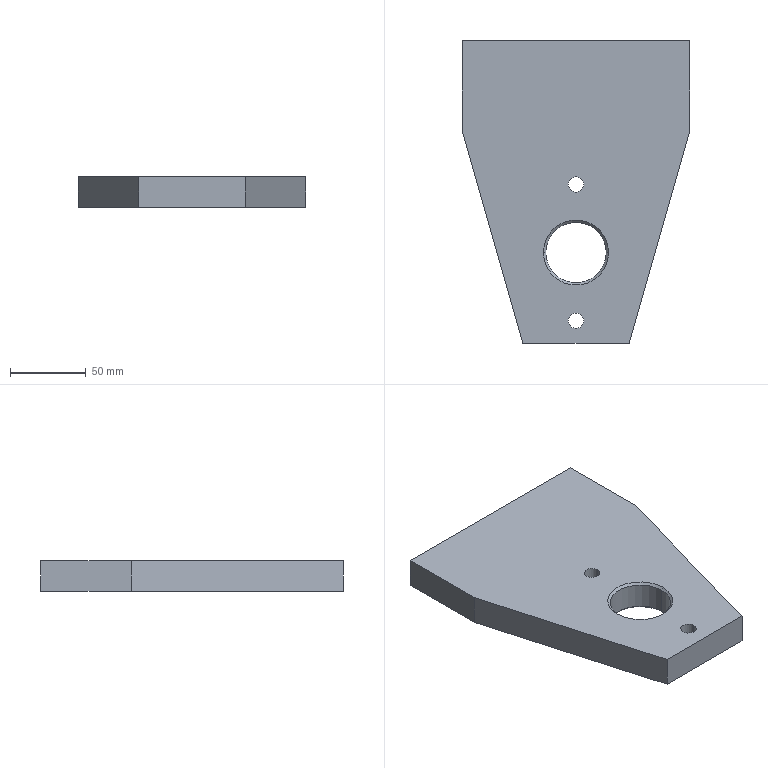Part | SolidWorks | features Chamfer 1, Extrusion 1, HoleWzd 1 | 1 solid | 18 faces | box 150 x 200 x 20 mm | volume 459309 mm3 | plane 8 | cylinder 6 | cone 4 | commonest cylinder face diameters 10.2 x4 40 x2
STEP:
#1=CARTESIAN_POINT('',(55.,-140.,18.5));
#2=VERTEX_POINT('',#1);
#3=CARTESIAN_POINT('',(95.,-140.,18.5));
#4=VERTEX_POINT('',#3);
#5=CARTESIAN_POINT('',(75.,-140.,18.5));
#6=DIRECTION('',(0.,0.,1.));
#7=DIRECTION('',(-1.,0.,0.));
#8=AXIS2_PLACEMENT_3D('',#5,#6,#7);
#9=CIRCLE('',#8,20.);
#10=EDGE_CURVE('',#2,#4,#9,.T.);
#11=ORIENTED_EDGE('',*,*,#10,.F.);
#12=CARTESIAN_POINT('',(53.5,-140.,20.));
#13=VERTEX_POINT('',#12);
#14=CARTESIAN_POINT('',(55.,-140.,18.5));
#15=DIRECTION('',(-0.7071,0.,0.7071));
#16=VECTOR('',#15,1000.);
#17=LINE('',#14,#16);
#18=EDGE_CURVE('',#2,#13,#17,.T.);
#19=ORIENTED_EDGE('',*,*,#18,.T.);
#20=CARTESIAN_POINT('',(96.5,-140.,20.));
#21=VERTEX_POINT('',#20);
#22=CARTESIAN_POINT('',(75.,-140.,20.));
#23=DIRECTION('',(0.,0.,-1.));
#24=DIRECTION('',(-1.,0.,0.));
#25=AXIS2_PLACEMENT_3D('',#22,#23,#24);
#26=CIRCLE('',#25,21.5);
#27=EDGE_CURVE('',#21,#13,#26,.T.);
#28=ORIENTED_EDGE('',*,*,#27,.F.);
#29=CARTESIAN_POINT('',(95.,-140.,18.5));
#30=DIRECTION('',(0.7071,0.,0.7071));
#31=VECTOR('',#30,1000.);
#32=LINE('',#29,#31);
#33=EDGE_CURVE('',#4,#21,#32,.T.);
#34=ORIENTED_EDGE('',*,*,#33,.F.);
#35=EDGE_LOOP('',(#11,#19,#28,#34));
#36=FACE_OUTER_BOUND('',#35,.T.);
#37=CARTESIAN_POINT('',(75.,-140.,18.5));
#38=DIRECTION('',(0.,0.,1.));
#39=DIRECTION('',(1.,0.,0.));
#40=AXIS2_PLACEMENT_3D('',#37,#38,#39);
#41=CONICAL_SURFACE('',#40,20.,0.7854);
#42=ADVANCED_FACE('',(#36),#41,.F.);
#43=CARTESIAN_POINT('',(95.,-140.,1.5));
#44=VERTEX_POINT('',#43);
#45=CARTESIAN_POINT('',(55.,-140.,1.5));
#46=VERTEX_POINT('',#45);
#47=CARTESIAN_POINT('',(75.,-140.,1.5));
#48=DIRECTION('',(0.,0.,-1.));
#49=DIRECTION('',(-1.,0.,0.));
#50=AXIS2_PLACEMENT_3D('',#47,#48,#49);
#51=CIRCLE('',#50,20.);
#52=EDGE_CURVE('',#44,#46,#51,.T.);
#53=ORIENTED_EDGE('',*,*,#52,.F.);
#54=CARTESIAN_POINT('',(96.5,-140.,0.));
#55=VERTEX_POINT('',#54);
#56=CARTESIAN_POINT('',(96.5,-140.,0.));
#57=DIRECTION('',(0.7071,0.,-0.7071));
#58=VECTOR('',#57,1000.);
#59=LINE('',#56,#58);
#60=EDGE_CURVE('',#44,#55,#59,.T.);
#61=ORIENTED_EDGE('',*,*,#60,.T.);
#62=CARTESIAN_POINT('',(53.5,-140.,0.));
#63=VERTEX_POINT('',#62);
#64=CARTESIAN_POINT('',(75.,-140.,0.));
#65=DIRECTION('',(0.,0.,1.));
#66=DIRECTION('',(-1.,0.,0.));
#67=AXIS2_PLACEMENT_3D('',#64,#65,#66);
#68=CIRCLE('',#67,21.5);
#69=EDGE_CURVE('',#63,#55,#68,.T.);
#70=ORIENTED_EDGE('',*,*,#69,.F.);
#71=CARTESIAN_POINT('',(53.5,-140.,0.));
#72=DIRECTION('',(-0.7071,0.,-0.7071));
#73=VECTOR('',#72,1000.);
#74=LINE('',#71,#73);
#75=EDGE_CURVE('',#46,#63,#74,.T.);
#76=ORIENTED_EDGE('',*,*,#75,.F.);
#77=EDGE_LOOP('',(#53,#61,#70,#76));
#78=FACE_OUTER_BOUND('',#77,.T.);
#79=CARTESIAN_POINT('',(75.,-140.,0.));
#80=DIRECTION('',(0.,0.,-1.));
#81=DIRECTION('',(-1.,0.,0.));
#82=AXIS2_PLACEMENT_3D('',#79,#80,#81);
#83=CONICAL_SURFACE('',#82,21.5,0.7854);
#84=ADVANCED_FACE('',(#78),#83,.F.);
#85=CARTESIAN_POINT('',(80.1,-95.,0.));
#86=VERTEX_POINT('',#85);
#87=CARTESIAN_POINT('',(69.9,-95.,0.));
#88=VERTEX_POINT('',#87);
#89=CARTESIAN_POINT('',(75.,-95.,0.));
#90=DIRECTION('',(0.,0.,-1.));
#91=DIRECTION('',(-1.,0.,0.));
#92=AXIS2_PLACEMENT_3D('',#89,#90,#91);
#93=CIRCLE('',#92,5.1);
#94=EDGE_CURVE('',#86,#88,#93,.T.);
#95=ORIENTED_EDGE('',*,*,#94,.T.);
#96=CARTESIAN_POINT('',(69.9,-95.,20.));
#97=VERTEX_POINT('',#96);
#98=CARTESIAN_POINT('',(69.9,-95.,20.));
#99=DIRECTION('',(0.,0.,1.));
#100=VECTOR('',#99,1000.);
#101=LINE('',#98,#100);
#102=EDGE_CURVE('',#88,#97,#101,.T.);
#103=ORIENTED_EDGE('',*,*,#102,.T.);
#104=CARTESIAN_POINT('',(80.1,-95.,20.));
#105=VERTEX_POINT('',#104);
#106=CARTESIAN_POINT('',(75.,-95.,20.));
#107=DIRECTION('',(0.,0.,1.));
#108=DIRECTION('',(1.,0.,0.));
#109=AXIS2_PLACEMENT_3D('',#106,#107,#108);
#110=CIRCLE('',#109,5.1);
#111=EDGE_CURVE('',#97,#105,#110,.T.);
#112=ORIENTED_EDGE('',*,*,#111,.T.);
#113=CARTESIAN_POINT('',(80.1,-95.,20.));
#114=DIRECTION('',(0.,0.,1.));
#115=VECTOR('',#114,1000.);
#116=LINE('',#113,#115);
#117=EDGE_CURVE('',#86,#105,#116,.T.);
#118=ORIENTED_EDGE('',*,*,#117,.F.);
#119=EDGE_LOOP('',(#95,#103,#112,#118));
#120=FACE_OUTER_BOUND('',#119,.T.);
#121=CARTESIAN_POINT('',(75.,-95.,20.));
#122=DIRECTION('',(0.,0.,1.));
#123=DIRECTION('',(1.,0.,0.));
#124=AXIS2_PLACEMENT_3D('',#121,#122,#123);
#125=CYLINDRICAL_SURFACE('',#124,5.1);
#126=ADVANCED_FACE('',(#120),#125,.F.);
#127=CARTESIAN_POINT('',(80.1,-185.,0.));
#128=VERTEX_POINT('',#127);
#129=CARTESIAN_POINT('',(69.9,-185.,0.));
#130=VERTEX_POINT('',#129);
#131=CARTESIAN_POINT('',(75.,-185.,0.));
#132=DIRECTION('',(0.,0.,-1.));
#133=DIRECTION('',(-1.,0.,0.));
#134=AXIS2_PLACEMENT_3D('',#131,#132,#133);
#135=CIRCLE('',#134,5.1);
#136=EDGE_CURVE('',#128,#130,#135,.T.);
#137=ORIENTED_EDGE('',*,*,#136,.T.);
#138=CARTESIAN_POINT('',(69.9,-185.,20.));
#139=VERTEX_POINT('',#138);
#140=CARTESIAN_POINT('',(69.9,-185.,20.));
#141=DIRECTION('',(0.,0.,1.));
#142=VECTOR('',#141,1000.);
#143=LINE('',#140,#142);
#144=EDGE_CURVE('',#130,#139,#143,.T.);
#145=ORIENTED_EDGE('',*,*,#144,.T.);
#146=CARTESIAN_POINT('',(80.1,-185.,20.));
#147=VERTEX_POINT('',#146);
#148=CARTESIAN_POINT('',(75.,-185.,20.));
#149=DIRECTION('',(0.,0.,1.));
#150=DIRECTION('',(1.,0.,0.));
#151=AXIS2_PLACEMENT_3D('',#148,#149,#150);
#152=CIRCLE('',#151,5.1);
#153=EDGE_CURVE('',#139,#147,#152,.T.);
#154=ORIENTED_EDGE('',*,*,#153,.T.);
#155=CARTESIAN_POINT('',(80.1,-185.,20.));
#156=DIRECTION('',(0.,0.,1.));
#157=VECTOR('',#156,1000.);
#158=LINE('',#155,#157);
#159=EDGE_CURVE('',#128,#147,#158,.T.);
#160=ORIENTED_EDGE('',*,*,#159,.F.);
#161=EDGE_LOOP('',(#137,#145,#154,#160));
#162=FACE_OUTER_BOUND('',#161,.T.);
#163=CARTESIAN_POINT('',(75.,-185.,20.));
#164=DIRECTION('',(0.,0.,1.));
#165=DIRECTION('',(1.,0.,0.));
#166=AXIS2_PLACEMENT_3D('',#163,#164,#165);
#167=CYLINDRICAL_SURFACE('',#166,5.1);
#168=ADVANCED_FACE('',(#162),#167,.F.);
#169=ORIENTED_EDGE('',*,*,#10,.T.);
#170=CARTESIAN_POINT('',(95.,-140.,20.));
#171=DIRECTION('',(0.,0.,-1.));
#172=VECTOR('',#171,1000.);
#173=LINE('',#170,#172);
#174=EDGE_CURVE('',#4,#44,#173,.T.);
#175=ORIENTED_EDGE('',*,*,#174,.T.);
#176=ORIENTED_EDGE('',*,*,#52,.T.);
#177=CARTESIAN_POINT('',(55.,-140.,20.));
#178=DIRECTION('',(0.,0.,-1.));
#179=VECTOR('',#178,1000.);
#180=LINE('',#177,#179);
#181=EDGE_CURVE('',#2,#46,#180,.T.);
#182=ORIENTED_EDGE('',*,*,#181,.F.);
#183=EDGE_LOOP('',(#169,#175,#176,#182));
#184=FACE_OUTER_BOUND('',#183,.T.);
#185=CARTESIAN_POINT('',(75.,-140.,20.));
#186=DIRECTION('',(0.,0.,-1.));
#187=DIRECTION('',(-1.,0.,0.));
#188=AXIS2_PLACEMENT_3D('',#185,#186,#187);
#189=CYLINDRICAL_SURFACE('',#188,20.);
#190=ADVANCED_FACE('',(#184),#189,.F.);
#191=ORIENTED_EDGE('',*,*,#27,.T.);
#192=CARTESIAN_POINT('',(75.,-140.,20.));
#193=DIRECTION('',(0.,0.,-1.));
#194=DIRECTION('',(-1.,0.,0.));
#195=AXIS2_PLACEMENT_3D('',#192,#193,#194);
#196=CIRCLE('',#195,21.5);
#197=EDGE_CURVE('',#13,#21,#196,.T.);
#198=ORIENTED_EDGE('',*,*,#197,.T.);
#199=EDGE_LOOP('',(#191,#198));
#200=FACE_BOUND('',#199,.T.);
#201=CARTESIAN_POINT('',(75.,-95.,20.));
#202=DIRECTION('',(0.,0.,1.));
#203=DIRECTION('',(1.,0.,0.));
#204=AXIS2_PLACEMENT_3D('',#201,#202,#203);
#205=CIRCLE('',#204,5.1);
#206=EDGE_CURVE('',#105,#97,#205,.T.);
#207=ORIENTED_EDGE('',*,*,#206,.F.);
#208=ORIENTED_EDGE('',*,*,#111,.F.);
#209=EDGE_LOOP('',(#207,#208));
#210=FACE_BOUND('',#209,.T.);
#211=CARTESIAN_POINT('',(0.,0.,20.));
#212=VERTEX_POINT('',#211);
#213=CARTESIAN_POINT('',(0.,-60.,20.));
#214=VERTEX_POINT('',#213);
#215=CARTESIAN_POINT('',(0.,-60.,20.));
#216=DIRECTION('',(0.,-1.,0.));
#217=VECTOR('',#216,1000.);
#218=LINE('',#215,#217);
#219=EDGE_CURVE('',#212,#214,#218,.T.);
#220=ORIENTED_EDGE('',*,*,#219,.T.);
#221=CARTESIAN_POINT('',(40.,-200.,20.));
#222=VERTEX_POINT('',#221);
#223=CARTESIAN_POINT('',(40.,-200.,20.));
#224=DIRECTION('',(0.2747,-0.9615,0.));
#225=VECTOR('',#224,1000.);
#226=LINE('',#223,#225);
#227=EDGE_CURVE('',#214,#222,#226,.T.);
#228=ORIENTED_EDGE('',*,*,#227,.T.);
#229=CARTESIAN_POINT('',(110.,-200.,20.));
#230=VERTEX_POINT('',#229);
#231=CARTESIAN_POINT('',(110.,-200.,20.));
#232=DIRECTION('',(1.,0.,0.));
#233=VECTOR('',#232,1000.);
#234=LINE('',#231,#233);
#235=EDGE_CURVE('',#222,#230,#234,.T.);
#236=ORIENTED_EDGE('',*,*,#235,.T.);
#237=CARTESIAN_POINT('',(150.,-60.,20.));
#238=VERTEX_POINT('',#237);
#239=CARTESIAN_POINT('',(150.,-60.,20.));
#240=DIRECTION('',(0.2747,0.9615,0.));
#241=VECTOR('',#240,1000.);
#242=LINE('',#239,#241);
#243=EDGE_CURVE('',#230,#238,#242,.T.);
#244=ORIENTED_EDGE('',*,*,#243,.T.);
#245=CARTESIAN_POINT('',(150.,0.,20.));
#246=VERTEX_POINT('',#245);
#247=CARTESIAN_POINT('',(150.,0.,20.));
#248=DIRECTION('',(0.,1.,0.));
#249=VECTOR('',#248,1000.);
#250=LINE('',#247,#249);
#251=EDGE_CURVE('',#238,#246,#250,.T.);
#252=ORIENTED_EDGE('',*,*,#251,.T.);
#253=CARTESIAN_POINT('',(0.,0.,20.));
#254=DIRECTION('',(-1.,0.,0.));
#255=VECTOR('',#254,1000.);
#256=LINE('',#253,#255);
#257=EDGE_CURVE('',#246,#212,#256,.T.);
#258=ORIENTED_EDGE('',*,*,#257,.T.);
#259=EDGE_LOOP('',(#220,#228,#236,#244,#252,#258));
#260=FACE_OUTER_BOUND('',#259,.T.);
#261=CARTESIAN_POINT('',(75.,-185.,20.));
#262=DIRECTION('',(0.,0.,1.));
#263=DIRECTION('',(1.,0.,0.));
#264=AXIS2_PLACEMENT_3D('',#261,#262,#263);
#265=CIRCLE('',#264,5.1);
#266=EDGE_CURVE('',#147,#139,#265,.T.);
#267=ORIENTED_EDGE('',*,*,#266,.F.);
#268=ORIENTED_EDGE('',*,*,#153,.F.);
#269=EDGE_LOOP('',(#267,#268));
#270=FACE_BOUND('',#269,.T.);
#271=CARTESIAN_POINT('',(0.,0.,20.));
#272=DIRECTION('',(0.,0.,-1.));
#273=DIRECTION('',(-1.,0.,0.));
#274=AXIS2_PLACEMENT_3D('',#271,#272,#273);
#275=PLANE('',#274);
#276=ADVANCED_FACE('',(#200,#210,#260,#270),#275,.F.);
#277=ORIENTED_EDGE('',*,*,#69,.T.);
#278=CARTESIAN_POINT('',(75.,-140.,0.));
#279=DIRECTION('',(0.,0.,1.));
#280=DIRECTION('',(-1.,0.,0.));
#281=AXIS2_PLACEMENT_3D('',#278,#279,#280);
#282=CIRCLE('',#281,21.5);
#283=EDGE_CURVE('',#55,#63,#282,.T.);
#284=ORIENTED_EDGE('',*,*,#283,.T.);
#285=EDGE_LOOP('',(#277,#284));
#286=FACE_BOUND('',#285,.T.);
#287=ORIENTED_EDGE('',*,*,#94,.F.);
#288=CARTESIAN_POINT('',(75.,-95.,0.));
#289=DIRECTION('',(0.,0.,-1.));
#290=DIRECTION('',(-1.,0.,0.));
#291=AXIS2_PLACEMENT_3D('',#288,#289,#290);
#292=CIRCLE('',#291,5.1);
#293=EDGE_CURVE('',#88,#86,#292,.T.);
#294=ORIENTED_EDGE('',*,*,#293,.F.);
#295=EDGE_LOOP('',(#287,#294));
#296=FACE_BOUND('',#295,.T.);
#297=ORIENTED_EDGE('',*,*,#136,.F.);
#298=CARTESIAN_POINT('',(75.,-185.,0.));
#299=DIRECTION('',(0.,0.,-1.));
#300=DIRECTION('',(-1.,0.,0.));
#301=AXIS2_PLACEMENT_3D('',#298,#299,#300);
#302=CIRCLE('',#301,5.1);
#303=EDGE_CURVE('',#130,#128,#302,.T.);
#304=ORIENTED_EDGE('',*,*,#303,.F.);
#305=EDGE_LOOP('',(#297,#304));
#306=FACE_BOUND('',#305,.T.);
#307=CARTESIAN_POINT('',(0.,0.,0.));
#308=VERTEX_POINT('',#307);
#309=CARTESIAN_POINT('',(0.,-60.,0.));
#310=VERTEX_POINT('',#309);
#311=CARTESIAN_POINT('',(0.,-60.,0.));
#312=DIRECTION('',(0.,-1.,0.));
#313=VECTOR('',#312,1000.);
#314=LINE('',#311,#313);
#315=EDGE_CURVE('',#308,#310,#314,.T.);
#316=ORIENTED_EDGE('',*,*,#315,.F.);
#317=CARTESIAN_POINT('',(150.,0.,0.));
#318=VERTEX_POINT('',#317);
#319=CARTESIAN_POINT('',(0.,0.,0.));
#320=DIRECTION('',(-1.,0.,0.));
#321=VECTOR('',#320,1000.);
#322=LINE('',#319,#321);
#323=EDGE_CURVE('',#318,#308,#322,.T.);
#324=ORIENTED_EDGE('',*,*,#323,.F.);
#325=CARTESIAN_POINT('',(150.,-60.,0.));
#326=VERTEX_POINT('',#325);
#327=CARTESIAN_POINT('',(150.,0.,0.));
#328=DIRECTION('',(0.,1.,0.));
#329=VECTOR('',#328,1000.);
#330=LINE('',#327,#329);
#331=EDGE_CURVE('',#326,#318,#330,.T.);
#332=ORIENTED_EDGE('',*,*,#331,.F.);
#333=CARTESIAN_POINT('',(110.,-200.,0.));
#334=VERTEX_POINT('',#333);
#335=CARTESIAN_POINT('',(150.,-60.,0.));
#336=DIRECTION('',(0.2747,0.9615,0.));
#337=VECTOR('',#336,1000.);
#338=LINE('',#335,#337);
#339=EDGE_CURVE('',#334,#326,#338,.T.);
#340=ORIENTED_EDGE('',*,*,#339,.F.);
#341=CARTESIAN_POINT('',(40.,-200.,0.));
#342=VERTEX_POINT('',#341);
#343=CARTESIAN_POINT('',(110.,-200.,0.));
#344=DIRECTION('',(1.,0.,0.));
#345=VECTOR('',#344,1000.);
#346=LINE('',#343,#345);
#347=EDGE_CURVE('',#342,#334,#346,.T.);
#348=ORIENTED_EDGE('',*,*,#347,.F.);
#349=CARTESIAN_POINT('',(40.,-200.,0.));
#350=DIRECTION('',(0.2747,-0.9615,0.));
#351=VECTOR('',#350,1000.);
#352=LINE('',#349,#351);
#353=EDGE_CURVE('',#310,#342,#352,.T.);
#354=ORIENTED_EDGE('',*,*,#353,.F.);
#355=EDGE_LOOP('',(#316,#324,#332,#340,#348,#354));
#356=FACE_OUTER_BOUND('',#355,.T.);
#357=CARTESIAN_POINT('',(0.,0.,0.));
#358=DIRECTION('',(0.,0.,-1.));
#359=DIRECTION('',(-1.,0.,0.));
#360=AXIS2_PLACEMENT_3D('',#357,#358,#359);
#361=PLANE('',#360);
#362=ADVANCED_FACE('',(#286,#296,#306,#356),#361,.T.);
#363=ORIENTED_EDGE('',*,*,#315,.T.);
#364=CARTESIAN_POINT('',(0.,-60.,20.));
#365=DIRECTION('',(0.,0.,-1.));
#366=VECTOR('',#365,1000.);
#367=LINE('',#364,#366);
#368=EDGE_CURVE('',#214,#310,#367,.T.);
#369=ORIENTED_EDGE('',*,*,#368,.F.);
#370=ORIENTED_EDGE('',*,*,#219,.F.);
#371=CARTESIAN_POINT('',(0.,0.,20.));
#372=DIRECTION('',(0.,0.,-1.));
#373=VECTOR('',#372,1000.);
#374=LINE('',#371,#373);
#375=EDGE_CURVE('',#212,#308,#374,.T.);
#376=ORIENTED_EDGE('',*,*,#375,.T.);
#377=EDGE_LOOP('',(#363,#369,#370,#376));
#378=FACE_OUTER_BOUND('',#377,.T.);
#379=CARTESIAN_POINT('',(0.,-60.,20.));
#380=DIRECTION('',(1.,0.,0.));
#381=DIRECTION('',(0.,0.,-1.));
#382=AXIS2_PLACEMENT_3D('',#379,#380,#381);
#383=PLANE('',#382);
#384=ADVANCED_FACE('',(#378),#383,.F.);
#385=ORIENTED_EDGE('',*,*,#353,.T.);
#386=CARTESIAN_POINT('',(40.,-200.,20.));
#387=DIRECTION('',(0.,0.,-1.));
#388=VECTOR('',#387,1000.);
#389=LINE('',#386,#388);
#390=EDGE_CURVE('',#222,#342,#389,.T.);
#391=ORIENTED_EDGE('',*,*,#390,.F.);
#392=ORIENTED_EDGE('',*,*,#227,.F.);
#393=ORIENTED_EDGE('',*,*,#368,.T.);
#394=EDGE_LOOP('',(#385,#391,#392,#393));
#395=FACE_OUTER_BOUND('',#394,.T.);
#396=CARTESIAN_POINT('',(40.,-200.,20.));
#397=DIRECTION('',(0.9615,0.2747,0.));
#398=DIRECTION('',(-0.2747,0.9615,0.));
#399=AXIS2_PLACEMENT_3D('',#396,#397,#398);
#400=PLANE('',#399);
#401=ADVANCED_FACE('',(#395),#400,.F.);
#402=ORIENTED_EDGE('',*,*,#347,.T.);
#403=CARTESIAN_POINT('',(110.,-200.,20.));
#404=DIRECTION('',(0.,0.,-1.));
#405=VECTOR('',#404,1000.);
#406=LINE('',#403,#405);
#407=EDGE_CURVE('',#230,#334,#406,.T.);
#408=ORIENTED_EDGE('',*,*,#407,.F.);
#409=ORIENTED_EDGE('',*,*,#235,.F.);
#410=ORIENTED_EDGE('',*,*,#390,.T.);
#411=EDGE_LOOP('',(#402,#408,#409,#410));
#412=FACE_OUTER_BOUND('',#411,.T.);
#413=CARTESIAN_POINT('',(110.,-200.,20.));
#414=DIRECTION('',(0.,1.,0.));
#415=DIRECTION('',(0.,0.,1.));
#416=AXIS2_PLACEMENT_3D('',#413,#414,#415);
#417=PLANE('',#416);
#418=ADVANCED_FACE('',(#412),#417,.F.);
#419=ORIENTED_EDGE('',*,*,#339,.T.);
#420=CARTESIAN_POINT('',(150.,-60.,20.));
#421=DIRECTION('',(0.,0.,-1.));
#422=VECTOR('',#421,1000.);
#423=LINE('',#420,#422);
#424=EDGE_CURVE('',#238,#326,#423,.T.);
#425=ORIENTED_EDGE('',*,*,#424,.F.);
#426=ORIENTED_EDGE('',*,*,#243,.F.);
#427=ORIENTED_EDGE('',*,*,#407,.T.);
#428=EDGE_LOOP('',(#419,#425,#426,#427));
#429=FACE_OUTER_BOUND('',#428,.T.);
#430=CARTESIAN_POINT('',(150.,-60.,20.));
#431=DIRECTION('',(-0.9615,0.2747,0.));
#432=DIRECTION('',(-0.2747,-0.9615,0.));
#433=AXIS2_PLACEMENT_3D('',#430,#431,#432);
#434=PLANE('',#433);
#435=ADVANCED_FACE('',(#429),#434,.F.);
#436=ORIENTED_EDGE('',*,*,#331,.T.);
#437=CARTESIAN_POINT('',(150.,0.,20.));
#438=DIRECTION('',(0.,0.,-1.));
#439=VECTOR('',#438,1000.);
#440=LINE('',#437,#439);
#441=EDGE_CURVE('',#246,#318,#440,.T.);
#442=ORIENTED_EDGE('',*,*,#441,.F.);
#443=ORIENTED_EDGE('',*,*,#251,.F.);
#444=ORIENTED_EDGE('',*,*,#424,.T.);
#445=EDGE_LOOP('',(#436,#442,#443,#444));
#446=FACE_OUTER_BOUND('',#445,.T.);
#447=CARTESIAN_POINT('',(150.,0.,20.));
#448=DIRECTION('',(-1.,0.,0.));
#449=DIRECTION('',(0.,0.,1.));
#450=AXIS2_PLACEMENT_3D('',#447,#448,#449);
#451=PLANE('',#450);
#452=ADVANCED_FACE('',(#446),#451,.F.);
#453=ORIENTED_EDGE('',*,*,#323,.T.);
#454=ORIENTED_EDGE('',*,*,#375,.F.);
#455=ORIENTED_EDGE('',*,*,#257,.F.);
#456=ORIENTED_EDGE('',*,*,#441,.T.);
#457=EDGE_LOOP('',(#453,#454,#455,#456));
#458=FACE_OUTER_BOUND('',#457,.T.);
#459=CARTESIAN_POINT('',(0.,0.,20.));
#460=DIRECTION('',(0.,-1.,0.));
#461=DIRECTION('',(0.,0.,-1.));
#462=AXIS2_PLACEMENT_3D('',#459,#460,#461);
#463=PLANE('',#462);
#464=ADVANCED_FACE('',(#458),#463,.F.);
#465=ORIENTED_EDGE('',*,*,#174,.F.);
#466=CARTESIAN_POINT('',(75.,-140.,18.5));
#467=DIRECTION('',(0.,0.,1.));
#468=DIRECTION('',(-1.,0.,0.));
#469=AXIS2_PLACEMENT_3D('',#466,#467,#468);
#470=CIRCLE('',#469,20.);
#471=EDGE_CURVE('',#4,#2,#470,.T.);
#472=ORIENTED_EDGE('',*,*,#471,.T.);
#473=ORIENTED_EDGE('',*,*,#181,.T.);
#474=CARTESIAN_POINT('',(75.,-140.,1.5));
#475=DIRECTION('',(0.,0.,-1.));
#476=DIRECTION('',(-1.,0.,0.));
#477=AXIS2_PLACEMENT_3D('',#474,#475,#476);
#478=CIRCLE('',#477,20.);
#479=EDGE_CURVE('',#46,#44,#478,.T.);
#480=ORIENTED_EDGE('',*,*,#479,.T.);
#481=EDGE_LOOP('',(#465,#472,#473,#480));
#482=FACE_OUTER_BOUND('',#481,.T.);
#483=CARTESIAN_POINT('',(75.,-140.,20.));
#484=DIRECTION('',(0.,0.,-1.));
#485=DIRECTION('',(-1.,0.,0.));
#486=AXIS2_PLACEMENT_3D('',#483,#484,#485);
#487=CYLINDRICAL_SURFACE('',#486,20.);
#488=ADVANCED_FACE('',(#482),#487,.F.);
#489=ORIENTED_EDGE('',*,*,#144,.F.);
#490=ORIENTED_EDGE('',*,*,#303,.T.);
#491=ORIENTED_EDGE('',*,*,#159,.T.);
#492=ORIENTED_EDGE('',*,*,#266,.T.);
#493=EDGE_LOOP('',(#489,#490,#491,#492));
#494=FACE_OUTER_BOUND('',#493,.T.);
#495=CARTESIAN_POINT('',(75.,-185.,20.));
#496=DIRECTION('',(0.,0.,1.));
#497=DIRECTION('',(1.,0.,0.));
#498=AXIS2_PLACEMENT_3D('',#495,#496,#497);
#499=CYLINDRICAL_SURFACE('',#498,5.1);
#500=ADVANCED_FACE('',(#494),#499,.F.);
#501=ORIENTED_EDGE('',*,*,#102,.F.);
#502=ORIENTED_EDGE('',*,*,#293,.T.);
#503=ORIENTED_EDGE('',*,*,#117,.T.);
#504=ORIENTED_EDGE('',*,*,#206,.T.);
#505=EDGE_LOOP('',(#501,#502,#503,#504));
#506=FACE_OUTER_BOUND('',#505,.T.);
#507=CARTESIAN_POINT('',(75.,-95.,20.));
#508=DIRECTION('',(0.,0.,1.));
#509=DIRECTION('',(1.,0.,0.));
#510=AXIS2_PLACEMENT_3D('',#507,#508,#509);
#511=CYLINDRICAL_SURFACE('',#510,5.1);
#512=ADVANCED_FACE('',(#506),#511,.F.);
#513=ORIENTED_EDGE('',*,*,#60,.F.);
#514=ORIENTED_EDGE('',*,*,#479,.F.);
#515=ORIENTED_EDGE('',*,*,#75,.T.);
#516=ORIENTED_EDGE('',*,*,#283,.F.);
#517=EDGE_LOOP('',(#513,#514,#515,#516));
#518=FACE_OUTER_BOUND('',#517,.T.);
#519=CARTESIAN_POINT('',(75.,-140.,0.));
#520=DIRECTION('',(0.,0.,-1.));
#521=DIRECTION('',(-1.,0.,0.));
#522=AXIS2_PLACEMENT_3D('',#519,#520,#521);
#523=CONICAL_SURFACE('',#522,21.5,0.7854);
#524=ADVANCED_FACE('',(#518),#523,.F.);
#525=ORIENTED_EDGE('',*,*,#18,.F.);
#526=ORIENTED_EDGE('',*,*,#471,.F.);
#527=ORIENTED_EDGE('',*,*,#33,.T.);
#528=ORIENTED_EDGE('',*,*,#197,.F.);
#529=EDGE_LOOP('',(#525,#526,#527,#528));
#530=FACE_OUTER_BOUND('',#529,.T.);
#531=CARTESIAN_POINT('',(75.,-140.,18.5));
#532=DIRECTION('',(0.,0.,1.));
#533=DIRECTION('',(1.,0.,0.));
#534=AXIS2_PLACEMENT_3D('',#531,#532,#533);
#535=CONICAL_SURFACE('',#534,20.,0.7854);
#536=ADVANCED_FACE('',(#530),#535,.F.);
#537=CLOSED_SHELL('',(#42,#84,#126,#168,#190,#276,#362,#384,#401,#418,#435,#452,#464,#488,#500,#512,#524,#536));
#538=MANIFOLD_SOLID_BREP('',#537);
#539=CARTESIAN_POINT('',(0.,0.,0.));
#540=DIRECTION('',(0.,0.,1.));
#541=DIRECTION('',(1.,0.,0.));
#542=AXIS2_PLACEMENT_3D('',#539,#540,#541);
#543=(LENGTH_UNIT()NAMED_UNIT(*)SI_UNIT(.MILLI.,.METRE.));
#544=UNCERTAINTY_MEASURE_WITH_UNIT(LENGTH_MEASURE(0.00001),#543,'','');
#545=(NAMED_UNIT(*)PLANE_ANGLE_UNIT()SI_UNIT($,.RADIAN.));
#546=(NAMED_UNIT(*)SI_UNIT($,.STERADIAN.)SOLID_ANGLE_UNIT());
#547=(GEOMETRIC_REPRESENTATION_CONTEXT(3)GLOBAL_UNCERTAINTY_ASSIGNED_CONTEXT((#544))GLOBAL_UNIT_ASSIGNED_CONTEXT((#543,#545,#546))REPRESENTATION_CONTEXT('',''));
#548=ADVANCED_BREP_SHAPE_REPRESENTATION('',(#538,#542),#547);